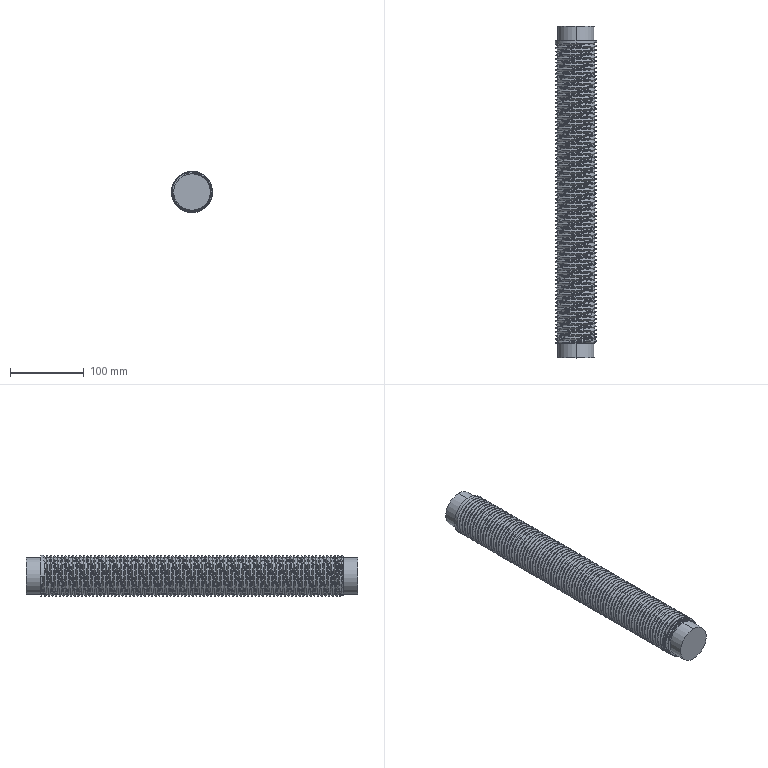Part | SolidWorks | features ICE 2, Extrusion 1, SweepThread 1 | 1 solid | 177 faces | box 56 x 450 x 56 mm | volume 978564 mm3 | cylinder 169 | plane 5 | spline 3 | commonest cylinder face diameters 56 x165 49.5 x4